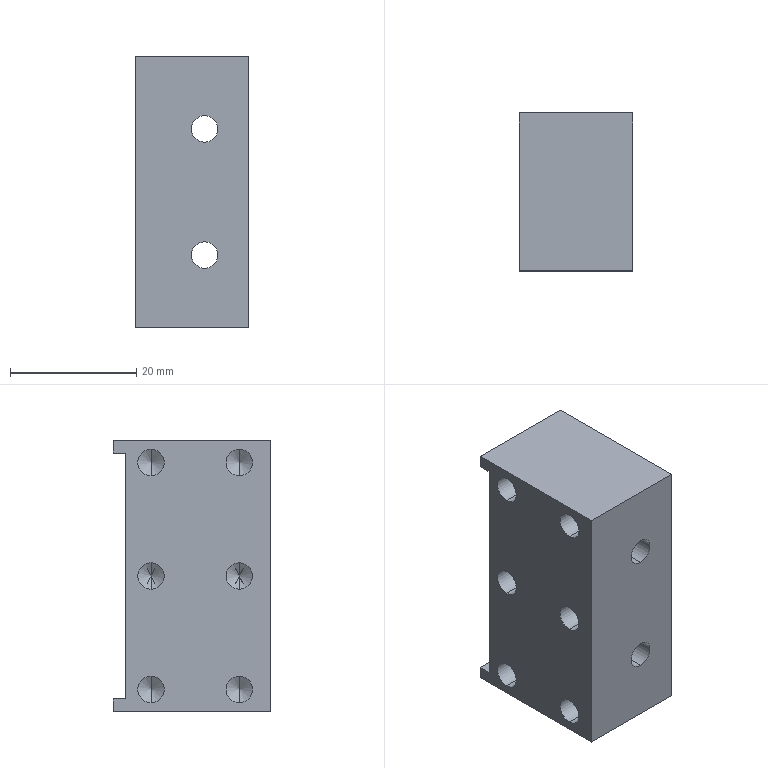Part | NX | features BREP 1 | 1 solid | 38 faces | box 18 x 25 x 43 mm | volume 16077 mm3 | cylinder 16 | cone 12 | plane 10 | commonest cylinder face diameters 4.2 x16
STEP:
#1=CARTESIAN_POINT('',(2.,23.,7.9));
#2=VERTEX_POINT('',#1);
#3=CARTESIAN_POINT('',(2.,0.,7.9));
#4=VERTEX_POINT('',#3);
#5=CARTESIAN_POINT('',(2.,23.,7.9));
#6=DIRECTION('',(0.,1.,0.));
#7=VECTOR('',#6,1000.);
#8=LINE('',#5,#7);
#9=EDGE_CURVE('',#2,#4,#8,.F.);
#10=ORIENTED_EDGE('',*,*,#9,.T.);
#11=CARTESIAN_POINT('',(2.,0.,12.1));
#12=VERTEX_POINT('',#11);
#13=CARTESIAN_POINT('',(2.,0.,10.));
#14=DIRECTION('',(0.,1.,0.));
#15=DIRECTION('',(0.,0.,1.));
#16=AXIS2_PLACEMENT_3D('',#13,#14,#15);
#17=CIRCLE('',#16,2.1);
#18=EDGE_CURVE('',#12,#4,#17,.T.);
#19=ORIENTED_EDGE('',*,*,#18,.F.);
#20=CARTESIAN_POINT('',(2.,23.,12.1));
#21=VERTEX_POINT('',#20);
#22=CARTESIAN_POINT('',(2.,23.,12.1));
#23=DIRECTION('',(0.,1.,0.));
#24=VECTOR('',#23,1000.);
#25=LINE('',#22,#24);
#26=EDGE_CURVE('',#21,#12,#25,.F.);
#27=ORIENTED_EDGE('',*,*,#26,.F.);
#28=CARTESIAN_POINT('',(2.,23.,10.));
#29=DIRECTION('',(0.,1.,0.));
#30=DIRECTION('',(0.,0.,1.));
#31=AXIS2_PLACEMENT_3D('',#28,#29,#30);
#32=CIRCLE('',#31,2.1);
#33=EDGE_CURVE('',#21,#2,#32,.T.);
#34=ORIENTED_EDGE('',*,*,#33,.T.);
#35=EDGE_LOOP('',(#10,#19,#27,#34));
#36=FACE_BOUND('',#35,.T.);
#37=CARTESIAN_POINT('',(2.,23.,10.));
#38=DIRECTION('',(0.,1.,0.));
#39=DIRECTION('',(0.,0.,1.));
#40=AXIS2_PLACEMENT_3D('',#37,#38,#39);
#41=CYLINDRICAL_SURFACE('',#40,2.1);
#42=ADVANCED_FACE('',(#36),#41,.F.);
#43=CARTESIAN_POINT('',(2.,23.,-12.1));
#44=VERTEX_POINT('',#43);
#45=CARTESIAN_POINT('',(2.,0.,-12.1));
#46=VERTEX_POINT('',#45);
#47=CARTESIAN_POINT('',(2.,23.,-12.1));
#48=DIRECTION('',(0.,1.,0.));
#49=VECTOR('',#48,1000.);
#50=LINE('',#47,#49);
#51=EDGE_CURVE('',#44,#46,#50,.F.);
#52=ORIENTED_EDGE('',*,*,#51,.T.);
#53=CARTESIAN_POINT('',(2.,0.,-7.9));
#54=VERTEX_POINT('',#53);
#55=CARTESIAN_POINT('',(2.,0.,-10.));
#56=DIRECTION('',(0.,1.,0.));
#57=DIRECTION('',(0.,0.,1.));
#58=AXIS2_PLACEMENT_3D('',#55,#56,#57);
#59=CIRCLE('',#58,2.1);
#60=EDGE_CURVE('',#54,#46,#59,.T.);
#61=ORIENTED_EDGE('',*,*,#60,.F.);
#62=CARTESIAN_POINT('',(2.,23.,-7.9));
#63=VERTEX_POINT('',#62);
#64=CARTESIAN_POINT('',(2.,23.,-7.9));
#65=DIRECTION('',(0.,1.,0.));
#66=VECTOR('',#65,1000.);
#67=LINE('',#64,#66);
#68=EDGE_CURVE('',#63,#54,#67,.F.);
#69=ORIENTED_EDGE('',*,*,#68,.F.);
#70=CARTESIAN_POINT('',(2.,23.,-10.));
#71=DIRECTION('',(0.,1.,0.));
#72=DIRECTION('',(0.,0.,1.));
#73=AXIS2_PLACEMENT_3D('',#70,#71,#72);
#74=CIRCLE('',#73,2.1);
#75=EDGE_CURVE('',#63,#44,#74,.T.);
#76=ORIENTED_EDGE('',*,*,#75,.T.);
#77=EDGE_LOOP('',(#52,#61,#69,#76));
#78=FACE_BOUND('',#77,.T.);
#79=CARTESIAN_POINT('',(2.,23.,-10.));
#80=DIRECTION('',(0.,1.,0.));
#81=DIRECTION('',(0.,0.,1.));
#82=AXIS2_PLACEMENT_3D('',#79,#80,#81);
#83=CYLINDRICAL_SURFACE('',#82,2.1);
#84=ADVANCED_FACE('',(#78),#83,.F.);
#85=CARTESIAN_POINT('',(-9.,5.,15.9));
#86=VERTEX_POINT('',#85);
#87=CARTESIAN_POINT('',(5.4,5.,15.9));
#88=VERTEX_POINT('',#87);
#89=CARTESIAN_POINT('',(-9.,5.,15.9));
#90=DIRECTION('',(-1.,0.,0.));
#91=VECTOR('',#90,1000.);
#92=LINE('',#89,#91);
#93=EDGE_CURVE('',#86,#88,#92,.F.);
#94=ORIENTED_EDGE('',*,*,#93,.T.);
#95=CARTESIAN_POINT('',(5.4,5.,20.1));
#96=VERTEX_POINT('',#95);
#97=CARTESIAN_POINT('',(5.4,5.,18.));
#98=DIRECTION('',(-1.,0.,0.));
#99=DIRECTION('',(0.,0.,1.));
#100=AXIS2_PLACEMENT_3D('',#97,#98,#99);
#101=CIRCLE('',#100,2.1);
#102=EDGE_CURVE('',#96,#88,#101,.T.);
#103=ORIENTED_EDGE('',*,*,#102,.F.);
#104=CARTESIAN_POINT('',(-9.,5.,20.1));
#105=VERTEX_POINT('',#104);
#106=CARTESIAN_POINT('',(-9.,5.,20.1));
#107=DIRECTION('',(-1.,0.,0.));
#108=VECTOR('',#107,1000.);
#109=LINE('',#106,#108);
#110=EDGE_CURVE('',#105,#96,#109,.F.);
#111=ORIENTED_EDGE('',*,*,#110,.F.);
#112=CARTESIAN_POINT('',(-9.,5.,18.));
#113=DIRECTION('',(-1.,0.,0.));
#114=DIRECTION('',(0.,0.,1.));
#115=AXIS2_PLACEMENT_3D('',#112,#113,#114);
#116=CIRCLE('',#115,2.1);
#117=EDGE_CURVE('',#105,#86,#116,.T.);
#118=ORIENTED_EDGE('',*,*,#117,.T.);
#119=EDGE_LOOP('',(#94,#103,#111,#118));
#120=FACE_BOUND('',#119,.T.);
#121=CARTESIAN_POINT('',(-9.,5.,18.));
#122=DIRECTION('',(-1.,0.,0.));
#123=DIRECTION('',(0.,0.,1.));
#124=AXIS2_PLACEMENT_3D('',#121,#122,#123);
#125=CYLINDRICAL_SURFACE('',#124,2.1);
#126=ADVANCED_FACE('',(#120),#125,.F.);
#127=CARTESIAN_POINT('',(6.662,5.,18.));
#128=VERTEX_POINT('',#127);
#129=CARTESIAN_POINT('',(5.4,5.,15.9));
#130=DIRECTION('',(-0.515,0.,-0.8572));
#131=VECTOR('',#130,1000.);
#132=LINE('',#129,#131);
#133=EDGE_CURVE('',#128,#88,#132,.T.);
#134=ORIENTED_EDGE('',*,*,#133,.F.);
#135=CARTESIAN_POINT('',(5.4,5.,20.1));
#136=DIRECTION('',(-0.515,0.,0.8572));
#137=VECTOR('',#136,1000.);
#138=LINE('',#135,#137);
#139=EDGE_CURVE('',#128,#96,#138,.T.);
#140=ORIENTED_EDGE('',*,*,#139,.T.);
#141=ORIENTED_EDGE('',*,*,#102,.T.);
#142=EDGE_LOOP('',(#134,#140,#141));
#143=FACE_BOUND('',#142,.T.);
#144=CARTESIAN_POINT('',(5.4,5.,18.));
#145=DIRECTION('',(-1.,0.,0.));
#146=DIRECTION('',(0.,0.,1.));
#147=AXIS2_PLACEMENT_3D('',#144,#145,#146);
#148=CONICAL_SURFACE('',#147,2.1,1.03);
#149=ADVANCED_FACE('',(#143),#148,.F.);
#150=CARTESIAN_POINT('',(-9.,5.,-2.1));
#151=VERTEX_POINT('',#150);
#152=CARTESIAN_POINT('',(5.4,5.,-2.1));
#153=VERTEX_POINT('',#152);
#154=CARTESIAN_POINT('',(-9.,5.,-2.1));
#155=DIRECTION('',(-1.,0.,0.));
#156=VECTOR('',#155,1000.);
#157=LINE('',#154,#156);
#158=EDGE_CURVE('',#151,#153,#157,.F.);
#159=ORIENTED_EDGE('',*,*,#158,.T.);
#160=CARTESIAN_POINT('',(5.4,5.,2.1));
#161=VERTEX_POINT('',#160);
#162=CARTESIAN_POINT('',(5.4,5.,0.));
#163=DIRECTION('',(-1.,0.,0.));
#164=DIRECTION('',(0.,0.,1.));
#165=AXIS2_PLACEMENT_3D('',#162,#163,#164);
#166=CIRCLE('',#165,2.1);
#167=EDGE_CURVE('',#161,#153,#166,.T.);
#168=ORIENTED_EDGE('',*,*,#167,.F.);
#169=CARTESIAN_POINT('',(-9.,5.,2.1));
#170=VERTEX_POINT('',#169);
#171=CARTESIAN_POINT('',(-9.,5.,2.1));
#172=DIRECTION('',(-1.,0.,0.));
#173=VECTOR('',#172,1000.);
#174=LINE('',#171,#173);
#175=EDGE_CURVE('',#170,#161,#174,.F.);
#176=ORIENTED_EDGE('',*,*,#175,.F.);
#177=CARTESIAN_POINT('',(-9.,5.,0.));
#178=DIRECTION('',(-1.,0.,0.));
#179=DIRECTION('',(0.,0.,1.));
#180=AXIS2_PLACEMENT_3D('',#177,#178,#179);
#181=CIRCLE('',#180,2.1);
#182=EDGE_CURVE('',#170,#151,#181,.T.);
#183=ORIENTED_EDGE('',*,*,#182,.T.);
#184=EDGE_LOOP('',(#159,#168,#176,#183));
#185=FACE_BOUND('',#184,.T.);
#186=CARTESIAN_POINT('',(-9.,5.,0.));
#187=DIRECTION('',(-1.,0.,0.));
#188=DIRECTION('',(0.,0.,1.));
#189=AXIS2_PLACEMENT_3D('',#186,#187,#188);
#190=CYLINDRICAL_SURFACE('',#189,2.1);
#191=ADVANCED_FACE('',(#185),#190,.F.);
#192=CARTESIAN_POINT('',(6.662,5.,0.));
#193=VERTEX_POINT('',#192);
#194=CARTESIAN_POINT('',(5.4,5.,-2.1));
#195=DIRECTION('',(-0.515,0.,-0.8572));
#196=VECTOR('',#195,1000.);
#197=LINE('',#194,#196);
#198=EDGE_CURVE('',#193,#153,#197,.T.);
#199=ORIENTED_EDGE('',*,*,#198,.F.);
#200=CARTESIAN_POINT('',(5.4,5.,2.1));
#201=DIRECTION('',(-0.515,0.,0.8572));
#202=VECTOR('',#201,1000.);
#203=LINE('',#200,#202);
#204=EDGE_CURVE('',#193,#161,#203,.T.);
#205=ORIENTED_EDGE('',*,*,#204,.T.);
#206=ORIENTED_EDGE('',*,*,#167,.T.);
#207=EDGE_LOOP('',(#199,#205,#206));
#208=FACE_BOUND('',#207,.T.);
#209=CARTESIAN_POINT('',(5.4,5.,0.));
#210=DIRECTION('',(-1.,0.,0.));
#211=DIRECTION('',(0.,0.,1.));
#212=AXIS2_PLACEMENT_3D('',#209,#210,#211);
#213=CONICAL_SURFACE('',#212,2.1,1.03);
#214=ADVANCED_FACE('',(#208),#213,.F.);
#215=CARTESIAN_POINT('',(-9.,5.,-20.1));
#216=VERTEX_POINT('',#215);
#217=CARTESIAN_POINT('',(5.4,5.,-20.1));
#218=VERTEX_POINT('',#217);
#219=CARTESIAN_POINT('',(-9.,5.,-20.1));
#220=DIRECTION('',(-1.,0.,0.));
#221=VECTOR('',#220,1000.);
#222=LINE('',#219,#221);
#223=EDGE_CURVE('',#216,#218,#222,.F.);
#224=ORIENTED_EDGE('',*,*,#223,.T.);
#225=CARTESIAN_POINT('',(5.4,5.,-15.9));
#226=VERTEX_POINT('',#225);
#227=CARTESIAN_POINT('',(5.4,5.,-18.));
#228=DIRECTION('',(-1.,0.,0.));
#229=DIRECTION('',(0.,0.,1.));
#230=AXIS2_PLACEMENT_3D('',#227,#228,#229);
#231=CIRCLE('',#230,2.1);
#232=EDGE_CURVE('',#226,#218,#231,.T.);
#233=ORIENTED_EDGE('',*,*,#232,.F.);
#234=CARTESIAN_POINT('',(-9.,5.,-15.9));
#235=VERTEX_POINT('',#234);
#236=CARTESIAN_POINT('',(-9.,5.,-15.9));
#237=DIRECTION('',(-1.,0.,0.));
#238=VECTOR('',#237,1000.);
#239=LINE('',#236,#238);
#240=EDGE_CURVE('',#235,#226,#239,.F.);
#241=ORIENTED_EDGE('',*,*,#240,.F.);
#242=CARTESIAN_POINT('',(-9.,5.,-18.));
#243=DIRECTION('',(-1.,0.,0.));
#244=DIRECTION('',(0.,0.,1.));
#245=AXIS2_PLACEMENT_3D('',#242,#243,#244);
#246=CIRCLE('',#245,2.1);
#247=EDGE_CURVE('',#235,#216,#246,.T.);
#248=ORIENTED_EDGE('',*,*,#247,.T.);
#249=EDGE_LOOP('',(#224,#233,#241,#248));
#250=FACE_BOUND('',#249,.T.);
#251=CARTESIAN_POINT('',(-9.,5.,-18.));
#252=DIRECTION('',(-1.,0.,0.));
#253=DIRECTION('',(0.,0.,1.));
#254=AXIS2_PLACEMENT_3D('',#251,#252,#253);
#255=CYLINDRICAL_SURFACE('',#254,2.1);
#256=ADVANCED_FACE('',(#250),#255,.F.);
#257=CARTESIAN_POINT('',(6.662,5.,-18.));
#258=VERTEX_POINT('',#257);
#259=CARTESIAN_POINT('',(5.4,5.,-20.1));
#260=DIRECTION('',(-0.515,0.,-0.8572));
#261=VECTOR('',#260,1000.);
#262=LINE('',#259,#261);
#263=EDGE_CURVE('',#258,#218,#262,.T.);
#264=ORIENTED_EDGE('',*,*,#263,.F.);
#265=CARTESIAN_POINT('',(5.4,5.,-15.9));
#266=DIRECTION('',(-0.515,0.,0.8572));
#267=VECTOR('',#266,1000.);
#268=LINE('',#265,#267);
#269=EDGE_CURVE('',#258,#226,#268,.T.);
#270=ORIENTED_EDGE('',*,*,#269,.T.);
#271=ORIENTED_EDGE('',*,*,#232,.T.);
#272=EDGE_LOOP('',(#264,#270,#271));
#273=FACE_BOUND('',#272,.T.);
#274=CARTESIAN_POINT('',(5.4,5.,-18.));
#275=DIRECTION('',(-1.,0.,0.));
#276=DIRECTION('',(0.,0.,1.));
#277=AXIS2_PLACEMENT_3D('',#274,#275,#276);
#278=CONICAL_SURFACE('',#277,2.1,1.03);
#279=ADVANCED_FACE('',(#273),#278,.F.);
#280=CARTESIAN_POINT('',(-9.,19.,15.9));
#281=VERTEX_POINT('',#280);
#282=CARTESIAN_POINT('',(5.4,19.,15.9));
#283=VERTEX_POINT('',#282);
#284=CARTESIAN_POINT('',(-9.,19.,15.9));
#285=DIRECTION('',(-1.,0.,0.));
#286=VECTOR('',#285,1000.);
#287=LINE('',#284,#286);
#288=EDGE_CURVE('',#281,#283,#287,.F.);
#289=ORIENTED_EDGE('',*,*,#288,.T.);
#290=CARTESIAN_POINT('',(5.4,19.,20.1));
#291=VERTEX_POINT('',#290);
#292=CARTESIAN_POINT('',(5.4,19.,18.));
#293=DIRECTION('',(-1.,0.,0.));
#294=DIRECTION('',(0.,0.,1.));
#295=AXIS2_PLACEMENT_3D('',#292,#293,#294);
#296=CIRCLE('',#295,2.1);
#297=EDGE_CURVE('',#291,#283,#296,.T.);
#298=ORIENTED_EDGE('',*,*,#297,.F.);
#299=CARTESIAN_POINT('',(-9.,19.,20.1));
#300=VERTEX_POINT('',#299);
#301=CARTESIAN_POINT('',(-9.,19.,20.1));
#302=DIRECTION('',(-1.,0.,0.));
#303=VECTOR('',#302,1000.);
#304=LINE('',#301,#303);
#305=EDGE_CURVE('',#300,#291,#304,.F.);
#306=ORIENTED_EDGE('',*,*,#305,.F.);
#307=CARTESIAN_POINT('',(-9.,19.,18.));
#308=DIRECTION('',(-1.,0.,0.));
#309=DIRECTION('',(0.,0.,1.));
#310=AXIS2_PLACEMENT_3D('',#307,#308,#309);
#311=CIRCLE('',#310,2.1);
#312=EDGE_CURVE('',#300,#281,#311,.T.);
#313=ORIENTED_EDGE('',*,*,#312,.T.);
#314=EDGE_LOOP('',(#289,#298,#306,#313));
#315=FACE_BOUND('',#314,.T.);
#316=CARTESIAN_POINT('',(-9.,19.,18.));
#317=DIRECTION('',(-1.,0.,0.));
#318=DIRECTION('',(0.,0.,1.));
#319=AXIS2_PLACEMENT_3D('',#316,#317,#318);
#320=CYLINDRICAL_SURFACE('',#319,2.1);
#321=ADVANCED_FACE('',(#315),#320,.F.);
#322=CARTESIAN_POINT('',(6.662,19.,18.));
#323=VERTEX_POINT('',#322);
#324=CARTESIAN_POINT('',(5.4,19.,15.9));
#325=DIRECTION('',(-0.515,0.,-0.8572));
#326=VECTOR('',#325,1000.);
#327=LINE('',#324,#326);
#328=EDGE_CURVE('',#323,#283,#327,.T.);
#329=ORIENTED_EDGE('',*,*,#328,.F.);
#330=CARTESIAN_POINT('',(5.4,19.,20.1));
#331=DIRECTION('',(-0.515,0.,0.8572));
#332=VECTOR('',#331,1000.);
#333=LINE('',#330,#332);
#334=EDGE_CURVE('',#323,#291,#333,.T.);
#335=ORIENTED_EDGE('',*,*,#334,.T.);
#336=ORIENTED_EDGE('',*,*,#297,.T.);
#337=EDGE_LOOP('',(#329,#335,#336));
#338=FACE_BOUND('',#337,.T.);
#339=CARTESIAN_POINT('',(5.4,19.,18.));
#340=DIRECTION('',(-1.,0.,0.));
#341=DIRECTION('',(0.,0.,1.));
#342=AXIS2_PLACEMENT_3D('',#339,#340,#341);
#343=CONICAL_SURFACE('',#342,2.1,1.03);
#344=ADVANCED_FACE('',(#338),#343,.F.);
#345=CARTESIAN_POINT('',(-9.,19.,-2.1));
#346=VERTEX_POINT('',#345);
#347=CARTESIAN_POINT('',(5.4,19.,-2.1));
#348=VERTEX_POINT('',#347);
#349=CARTESIAN_POINT('',(-9.,19.,-2.1));
#350=DIRECTION('',(-1.,0.,0.));
#351=VECTOR('',#350,1000.);
#352=LINE('',#349,#351);
#353=EDGE_CURVE('',#346,#348,#352,.F.);
#354=ORIENTED_EDGE('',*,*,#353,.T.);
#355=CARTESIAN_POINT('',(5.4,19.,2.1));
#356=VERTEX_POINT('',#355);
#357=CARTESIAN_POINT('',(5.4,19.,0.));
#358=DIRECTION('',(-1.,0.,0.));
#359=DIRECTION('',(0.,0.,1.));
#360=AXIS2_PLACEMENT_3D('',#357,#358,#359);
#361=CIRCLE('',#360,2.1);
#362=EDGE_CURVE('',#356,#348,#361,.T.);
#363=ORIENTED_EDGE('',*,*,#362,.F.);
#364=CARTESIAN_POINT('',(-9.,19.,2.1));
#365=VERTEX_POINT('',#364);
#366=CARTESIAN_POINT('',(-9.,19.,2.1));
#367=DIRECTION('',(-1.,0.,0.));
#368=VECTOR('',#367,1000.);
#369=LINE('',#366,#368);
#370=EDGE_CURVE('',#365,#356,#369,.F.);
#371=ORIENTED_EDGE('',*,*,#370,.F.);
#372=CARTESIAN_POINT('',(-9.,19.,0.));
#373=DIRECTION('',(-1.,0.,0.));
#374=DIRECTION('',(0.,0.,1.));
#375=AXIS2_PLACEMENT_3D('',#372,#373,#374);
#376=CIRCLE('',#375,2.1);
#377=EDGE_CURVE('',#365,#346,#376,.T.);
#378=ORIENTED_EDGE('',*,*,#377,.T.);
#379=EDGE_LOOP('',(#354,#363,#371,#378));
#380=FACE_BOUND('',#379,.T.);
#381=CARTESIAN_POINT('',(-9.,19.,0.));
#382=DIRECTION('',(-1.,0.,0.));
#383=DIRECTION('',(0.,0.,1.));
#384=AXIS2_PLACEMENT_3D('',#381,#382,#383);
#385=CYLINDRICAL_SURFACE('',#384,2.1);
#386=ADVANCED_FACE('',(#380),#385,.F.);
#387=CARTESIAN_POINT('',(6.662,19.,0.));
#388=VERTEX_POINT('',#387);
#389=CARTESIAN_POINT('',(5.4,19.,-2.1));
#390=DIRECTION('',(-0.515,0.,-0.8572));
#391=VECTOR('',#390,1000.);
#392=LINE('',#389,#391);
#393=EDGE_CURVE('',#388,#348,#392,.T.);
#394=ORIENTED_EDGE('',*,*,#393,.F.);
#395=CARTESIAN_POINT('',(5.4,19.,2.1));
#396=DIRECTION('',(-0.515,0.,0.8572));
#397=VECTOR('',#396,1000.);
#398=LINE('',#395,#397);
#399=EDGE_CURVE('',#388,#356,#398,.T.);
#400=ORIENTED_EDGE('',*,*,#399,.T.);
#401=ORIENTED_EDGE('',*,*,#362,.T.);
#402=EDGE_LOOP('',(#394,#400,#401));
#403=FACE_BOUND('',#402,.T.);
#404=CARTESIAN_POINT('',(5.4,19.,0.));
#405=DIRECTION('',(-1.,0.,0.));
#406=DIRECTION('',(0.,0.,1.));
#407=AXIS2_PLACEMENT_3D('',#404,#405,#406);
#408=CONICAL_SURFACE('',#407,2.1,1.03);
#409=ADVANCED_FACE('',(#403),#408,.F.);
#410=CARTESIAN_POINT('',(-9.,19.,-20.1));
#411=VERTEX_POINT('',#410);
#412=CARTESIAN_POINT('',(5.4,19.,-20.1));
#413=VERTEX_POINT('',#412);
#414=CARTESIAN_POINT('',(-9.,19.,-20.1));
#415=DIRECTION('',(-1.,0.,0.));
#416=VECTOR('',#415,1000.);
#417=LINE('',#414,#416);
#418=EDGE_CURVE('',#411,#413,#417,.F.);
#419=ORIENTED_EDGE('',*,*,#418,.T.);
#420=CARTESIAN_POINT('',(5.4,19.,-15.9));
#421=VERTEX_POINT('',#420);
#422=CARTESIAN_POINT('',(5.4,19.,-18.));
#423=DIRECTION('',(-1.,0.,0.));
#424=DIRECTION('',(0.,0.,1.));
#425=AXIS2_PLACEMENT_3D('',#422,#423,#424);
#426=CIRCLE('',#425,2.1);
#427=EDGE_CURVE('',#421,#413,#426,.T.);
#428=ORIENTED_EDGE('',*,*,#427,.F.);
#429=CARTESIAN_POINT('',(-9.,19.,-15.9));
#430=VERTEX_POINT('',#429);
#431=CARTESIAN_POINT('',(-9.,19.,-15.9));
#432=DIRECTION('',(-1.,0.,0.));
#433=VECTOR('',#432,1000.);
#434=LINE('',#431,#433);
#435=EDGE_CURVE('',#430,#421,#434,.F.);
#436=ORIENTED_EDGE('',*,*,#435,.F.);
#437=CARTESIAN_POINT('',(-9.,19.,-18.));
#438=DIRECTION('',(-1.,0.,0.));
#439=DIRECTION('',(0.,0.,1.));
#440=AXIS2_PLACEMENT_3D('',#437,#438,#439);
#441=CIRCLE('',#440,2.1);
#442=EDGE_CURVE('',#430,#411,#441,.T.);
#443=ORIENTED_EDGE('',*,*,#442,.T.);
#444=EDGE_LOOP('',(#419,#428,#436,#443));
#445=FACE_BOUND('',#444,.T.);
#446=CARTESIAN_POINT('',(-9.,19.,-18.));
#447=DIRECTION('',(-1.,0.,0.));
#448=DIRECTION('',(0.,0.,1.));
#449=AXIS2_PLACEMENT_3D('',#446,#447,#448);
#450=CYLINDRICAL_SURFACE('',#449,2.1);
#451=ADVANCED_FACE('',(#445),#450,.F.);
#452=CARTESIAN_POINT('',(6.662,19.,-18.));
#453=VERTEX_POINT('',#452);
#454=CARTESIAN_POINT('',(5.4,19.,-20.1));
#455=DIRECTION('',(-0.515,0.,-0.8572));
#456=VECTOR('',#455,1000.);
#457=LINE('',#454,#456);
#458=EDGE_CURVE('',#453,#413,#457,.T.);
#459=ORIENTED_EDGE('',*,*,#458,.F.);
#460=CARTESIAN_POINT('',(5.4,19.,-15.9));
#461=DIRECTION('',(-0.515,0.,0.8572));
#462=VECTOR('',#461,1000.);
#463=LINE('',#460,#462);
#464=EDGE_CURVE('',#453,#421,#463,.T.);
#465=ORIENTED_EDGE('',*,*,#464,.T.);
#466=ORIENTED_EDGE('',*,*,#427,.T.);
#467=EDGE_LOOP('',(#459,#465,#466));
#468=FACE_BOUND('',#467,.T.);
#469=CARTESIAN_POINT('',(5.4,19.,-18.));
#470=DIRECTION('',(-1.,0.,0.));
#471=DIRECTION('',(0.,0.,1.));
#472=AXIS2_PLACEMENT_3D('',#469,#470,#471);
#473=CONICAL_SURFACE('',#472,2.1,1.03);
#474=ADVANCED_FACE('',(#468),#473,.F.);
#475=CARTESIAN_POINT('',(-9.,23.,-19.5));
#476=VERTEX_POINT('',#475);
#477=CARTESIAN_POINT('',(-9.,23.,19.5));
#478=VERTEX_POINT('',#477);
#479=CARTESIAN_POINT('',(-9.,23.,19.5));
#480=DIRECTION('',(0.,0.,1.));
#481=VECTOR('',#480,1000.);
#482=LINE('',#479,#481);
#483=EDGE_CURVE('',#476,#478,#482,.T.);
#484=ORIENTED_EDGE('',*,*,#483,.T.);
#485=CARTESIAN_POINT('',(9.,23.,19.5));
#486=VERTEX_POINT('',#485);
#487=CARTESIAN_POINT('',(9.,23.,19.5));
#488=DIRECTION('',(1.,0.,0.));
#489=VECTOR('',#488,1000.);
#490=LINE('',#487,#489);
#491=EDGE_CURVE('',#478,#486,#490,.T.);
#492=ORIENTED_EDGE('',*,*,#491,.T.);
#493=CARTESIAN_POINT('',(9.,23.,-19.5));
#494=VERTEX_POINT('',#493);
#495=CARTESIAN_POINT('',(9.,23.,19.5));
#496=DIRECTION('',(0.,0.,-1.));
#497=VECTOR('',#496,1000.);
#498=LINE('',#495,#497);
#499=EDGE_CURVE('',#486,#494,#498,.T.);
#500=ORIENTED_EDGE('',*,*,#499,.T.);
#501=CARTESIAN_POINT('',(9.,23.,-19.5));
#502=DIRECTION('',(-1.,0.,0.));
#503=VECTOR('',#502,1000.);
#504=LINE('',#501,#503);
#505=EDGE_CURVE('',#494,#476,#504,.T.);
#506=ORIENTED_EDGE('',*,*,#505,.T.);
#507=EDGE_LOOP('',(#484,#492,#500,#506));
#508=FACE_BOUND('',#507,.T.);
#509=ORIENTED_EDGE('',*,*,#75,.F.);
#510=CARTESIAN_POINT('',(2.,23.,-10.));
#511=DIRECTION('',(0.,1.,0.));
#512=DIRECTION('',(0.,0.,1.));
#513=AXIS2_PLACEMENT_3D('',#510,#511,#512);
#514=CIRCLE('',#513,2.1);
#515=EDGE_CURVE('',#44,#63,#514,.T.);
#516=ORIENTED_EDGE('',*,*,#515,.F.);
#517=EDGE_LOOP('',(#509,#516));
#518=FACE_BOUND('',#517,.T.);
#519=ORIENTED_EDGE('',*,*,#33,.F.);
#520=CARTESIAN_POINT('',(2.,23.,10.));
#521=DIRECTION('',(0.,1.,0.));
#522=DIRECTION('',(0.,0.,1.));
#523=AXIS2_PLACEMENT_3D('',#520,#521,#522);
#524=CIRCLE('',#523,2.1);
#525=EDGE_CURVE('',#2,#21,#524,.T.);
#526=ORIENTED_EDGE('',*,*,#525,.F.);
#527=EDGE_LOOP('',(#519,#526));
#528=FACE_BOUND('',#527,.T.);
#529=CARTESIAN_POINT('',(0.,23.,0.));
#530=DIRECTION('',(0.,1.,0.));
#531=DIRECTION('',(0.,0.,1.));
#532=AXIS2_PLACEMENT_3D('',#529,#530,#531);
#533=PLANE('',#532);
#534=ADVANCED_FACE('',(#508,#518,#528),#533,.T.);
#535=CARTESIAN_POINT('',(-9.,25.,19.5));
#536=VERTEX_POINT('',#535);
#537=CARTESIAN_POINT('',(9.,25.,19.5));
#538=VERTEX_POINT('',#537);
#539=CARTESIAN_POINT('',(9.,25.,19.5));
#540=DIRECTION('',(1.,0.,0.));
#541=VECTOR('',#540,1000.);
#542=LINE('',#539,#541);
#543=EDGE_CURVE('',#536,#538,#542,.T.);
#544=ORIENTED_EDGE('',*,*,#543,.T.);
#545=CARTESIAN_POINT('',(9.,23.,19.5));
#546=DIRECTION('',(0.,1.,0.));
#547=VECTOR('',#546,1000.);
#548=LINE('',#545,#547);
#549=EDGE_CURVE('',#486,#538,#548,.T.);
#550=ORIENTED_EDGE('',*,*,#549,.F.);
#551=ORIENTED_EDGE('',*,*,#491,.F.);
#552=CARTESIAN_POINT('',(-9.,23.,19.5));
#553=DIRECTION('',(0.,1.,0.));
#554=VECTOR('',#553,1000.);
#555=LINE('',#552,#554);
#556=EDGE_CURVE('',#478,#536,#555,.T.);
#557=ORIENTED_EDGE('',*,*,#556,.T.);
#558=EDGE_LOOP('',(#544,#550,#551,#557));
#559=FACE_BOUND('',#558,.T.);
#560=CARTESIAN_POINT('',(9.,23.,19.5));
#561=DIRECTION('',(0.,0.,1.));
#562=DIRECTION('',(1.,0.,0.));
#563=AXIS2_PLACEMENT_3D('',#560,#561,#562);
#564=PLANE('',#563);
#565=ADVANCED_FACE('',(#559),#564,.F.);
#566=CARTESIAN_POINT('',(9.,25.,-19.5));
#567=VERTEX_POINT('',#566);
#568=CARTESIAN_POINT('',(-9.,25.,-19.5));
#569=VERTEX_POINT('',#568);
#570=CARTESIAN_POINT('',(9.,25.,-19.5));
#571=DIRECTION('',(-1.,0.,0.));
#572=VECTOR('',#571,1000.);
#573=LINE('',#570,#572);
#574=EDGE_CURVE('',#567,#569,#573,.T.);
#575=ORIENTED_EDGE('',*,*,#574,.T.);
#576=CARTESIAN_POINT('',(-9.,23.,-19.5));
#577=DIRECTION('',(0.,1.,0.));
#578=VECTOR('',#577,1000.);
#579=LINE('',#576,#578);
#580=EDGE_CURVE('',#476,#569,#579,.T.);
#581=ORIENTED_EDGE('',*,*,#580,.F.);
#582=ORIENTED_EDGE('',*,*,#505,.F.);
#583=CARTESIAN_POINT('',(9.,23.,-19.5));
#584=DIRECTION('',(0.,1.,0.));
#585=VECTOR('',#584,1000.);
#586=LINE('',#583,#585);
#587=EDGE_CURVE('',#494,#567,#586,.T.);
#588=ORIENTED_EDGE('',*,*,#587,.T.);
#589=EDGE_LOOP('',(#575,#581,#582,#588));
#590=FACE_BOUND('',#589,.T.);
#591=CARTESIAN_POINT('',(9.,23.,-19.5));
#592=DIRECTION('',(0.,0.,-1.));
#593=DIRECTION('',(-1.,0.,0.));
#594=AXIS2_PLACEMENT_3D('',#591,#592,#593);
#595=PLANE('',#594);
#596=ADVANCED_FACE('',(#590),#595,.F.);
#597=CARTESIAN_POINT('',(9.,0.,21.5));
#598=VERTEX_POINT('',#597);
#599=CARTESIAN_POINT('',(9.,0.,-21.5));
#600=VERTEX_POINT('',#599);
#601=CARTESIAN_POINT('',(9.,0.,21.5));
#602=DIRECTION('',(0.,0.,-1.));
#603=VECTOR('',#602,1000.);
#604=LINE('',#601,#603);
#605=EDGE_CURVE('',#598,#600,#604,.T.);
#606=ORIENTED_EDGE('',*,*,#605,.F.);
#607=CARTESIAN_POINT('',(-9.,0.,21.5));
#608=VERTEX_POINT('',#607);
#609=CARTESIAN_POINT('',(-9.,0.,21.5));
#610=DIRECTION('',(1.,0.,0.));
#611=VECTOR('',#610,1000.);
#612=LINE('',#609,#611);
#613=EDGE_CURVE('',#608,#598,#612,.T.);
#614=ORIENTED_EDGE('',*,*,#613,.F.);
#615=CARTESIAN_POINT('',(-9.,0.,-21.5));
#616=VERTEX_POINT('',#615);
#617=CARTESIAN_POINT('',(-9.,0.,21.5));
#618=DIRECTION('',(0.,0.,1.));
#619=VECTOR('',#618,1000.);
#620=LINE('',#617,#619);
#621=EDGE_CURVE('',#616,#608,#620,.T.);
#622=ORIENTED_EDGE('',*,*,#621,.F.);
#623=CARTESIAN_POINT('',(-9.,0.,-21.5));
#624=DIRECTION('',(-1.,0.,0.));
#625=VECTOR('',#624,1000.);
#626=LINE('',#623,#625);
#627=EDGE_CURVE('',#600,#616,#626,.T.);
#628=ORIENTED_EDGE('',*,*,#627,.F.);
#629=EDGE_LOOP('',(#606,#614,#622,#628));
#630=FACE_BOUND('',#629,.T.);
#631=ORIENTED_EDGE('',*,*,#60,.T.);
#632=CARTESIAN_POINT('',(2.,0.,-10.));
#633=DIRECTION('',(0.,1.,0.));
#634=DIRECTION('',(0.,0.,1.));
#635=AXIS2_PLACEMENT_3D('',#632,#633,#634);
#636=CIRCLE('',#635,2.1);
#637=EDGE_CURVE('',#46,#54,#636,.T.);
#638=ORIENTED_EDGE('',*,*,#637,.T.);
#639=EDGE_LOOP('',(#631,#638));
#640=FACE_BOUND('',#639,.T.);
#641=ORIENTED_EDGE('',*,*,#18,.T.);
#642=CARTESIAN_POINT('',(2.,0.,10.));
#643=DIRECTION('',(0.,1.,0.));
#644=DIRECTION('',(0.,0.,1.));
#645=AXIS2_PLACEMENT_3D('',#642,#643,#644);
#646=CIRCLE('',#645,2.1);
#647=EDGE_CURVE('',#4,#12,#646,.T.);
#648=ORIENTED_EDGE('',*,*,#647,.T.);
#649=EDGE_LOOP('',(#641,#648));
#650=FACE_BOUND('',#649,.T.);
#651=CARTESIAN_POINT('',(0.,0.,0.));
#652=DIRECTION('',(0.,-1.,0.));
#653=DIRECTION('',(0.,0.,-1.));
#654=AXIS2_PLACEMENT_3D('',#651,#652,#653);
#655=PLANE('',#654);
#656=ADVANCED_FACE('',(#630,#640,#650),#655,.T.);
#657=CARTESIAN_POINT('',(9.,25.,21.5));
#658=VERTEX_POINT('',#657);
#659=CARTESIAN_POINT('',(9.,25.,21.5));
#660=DIRECTION('',(0.,0.,-1.));
#661=VECTOR('',#660,1000.);
#662=LINE('',#659,#661);
#663=EDGE_CURVE('',#658,#538,#662,.T.);
#664=ORIENTED_EDGE('',*,*,#663,.T.);
#665=ORIENTED_EDGE('',*,*,#543,.F.);
#666=CARTESIAN_POINT('',(-9.,25.,21.5));
#667=VERTEX_POINT('',#666);
#668=CARTESIAN_POINT('',(-9.,25.,21.5));
#669=DIRECTION('',(0.,0.,1.));
#670=VECTOR('',#669,1000.);
#671=LINE('',#668,#670);
#672=EDGE_CURVE('',#536,#667,#671,.T.);
#673=ORIENTED_EDGE('',*,*,#672,.T.);
#674=CARTESIAN_POINT('',(-9.,25.,21.5));
#675=DIRECTION('',(1.,0.,0.));
#676=VECTOR('',#675,1000.);
#677=LINE('',#674,#676);
#678=EDGE_CURVE('',#667,#658,#677,.T.);
#679=ORIENTED_EDGE('',*,*,#678,.T.);
#680=EDGE_LOOP('',(#664,#665,#673,#679));
#681=FACE_BOUND('',#680,.T.);
#682=CARTESIAN_POINT('',(0.,25.,0.));
#683=DIRECTION('',(0.,-1.,0.));
#684=DIRECTION('',(0.,0.,-1.));
#685=AXIS2_PLACEMENT_3D('',#682,#683,#684);
#686=PLANE('',#685);
#687=ADVANCED_FACE('',(#681),#686,.F.);
#688=ORIENTED_EDGE('',*,*,#613,.T.);
#689=CARTESIAN_POINT('',(9.,25.,21.5));
#690=DIRECTION('',(0.,-1.,0.));
#691=VECTOR('',#690,1000.);
#692=LINE('',#689,#691);
#693=EDGE_CURVE('',#658,#598,#692,.T.);
#694=ORIENTED_EDGE('',*,*,#693,.F.);
#695=ORIENTED_EDGE('',*,*,#678,.F.);
#696=CARTESIAN_POINT('',(-9.,25.,21.5));
#697=DIRECTION('',(0.,-1.,0.));
#698=VECTOR('',#697,1000.);
#699=LINE('',#696,#698);
#700=EDGE_CURVE('',#667,#608,#699,.T.);
#701=ORIENTED_EDGE('',*,*,#700,.T.);
#702=EDGE_LOOP('',(#688,#694,#695,#701));
#703=FACE_BOUND('',#702,.T.);
#704=CARTESIAN_POINT('',(-9.,25.,21.5));
#705=DIRECTION('',(0.,0.,-1.));
#706=DIRECTION('',(-1.,0.,0.));
#707=AXIS2_PLACEMENT_3D('',#704,#705,#706);
#708=PLANE('',#707);
#709=ADVANCED_FACE('',(#703),#708,.F.);
#710=ORIENTED_EDGE('',*,*,#483,.F.);
#711=ORIENTED_EDGE('',*,*,#580,.T.);
#712=CARTESIAN_POINT('',(-9.,25.,-21.5));
#713=VERTEX_POINT('',#712);
#714=CARTESIAN_POINT('',(-9.,25.,21.5));
#715=DIRECTION('',(0.,0.,1.));
#716=VECTOR('',#715,1000.);
#717=LINE('',#714,#716);
#718=EDGE_CURVE('',#713,#569,#717,.T.);
#719=ORIENTED_EDGE('',*,*,#718,.F.);
#720=CARTESIAN_POINT('',(-9.,25.,-21.5));
#721=DIRECTION('',(0.,-1.,0.));
#722=VECTOR('',#721,1000.);
#723=LINE('',#720,#722);
#724=EDGE_CURVE('',#713,#616,#723,.T.);
#725=ORIENTED_EDGE('',*,*,#724,.T.);
#726=ORIENTED_EDGE('',*,*,#621,.T.);
#727=ORIENTED_EDGE('',*,*,#700,.F.);
#728=ORIENTED_EDGE('',*,*,#672,.F.);
#729=ORIENTED_EDGE('',*,*,#556,.F.);
#730=EDGE_LOOP('',(#710,#711,#719,#725,#726,#727,#728,#729));
#731=FACE_BOUND('',#730,.T.);
#732=ORIENTED_EDGE('',*,*,#442,.F.);
#733=CARTESIAN_POINT('',(-9.,19.,-18.));
#734=DIRECTION('',(-1.,0.,0.));
#735=DIRECTION('',(0.,0.,1.));
#736=AXIS2_PLACEMENT_3D('',#733,#734,#735);
#737=CIRCLE('',#736,2.1);
#738=EDGE_CURVE('',#411,#430,#737,.T.);
#739=ORIENTED_EDGE('',*,*,#738,.F.);
#740=EDGE_LOOP('',(#732,#739));
#741=FACE_BOUND('',#740,.T.);
#742=ORIENTED_EDGE('',*,*,#377,.F.);
#743=CARTESIAN_POINT('',(-9.,19.,0.));
#744=DIRECTION('',(-1.,0.,0.));
#745=DIRECTION('',(0.,0.,1.));
#746=AXIS2_PLACEMENT_3D('',#743,#744,#745);
#747=CIRCLE('',#746,2.1);
#748=EDGE_CURVE('',#346,#365,#747,.T.);
#749=ORIENTED_EDGE('',*,*,#748,.F.);
#750=EDGE_LOOP('',(#742,#749));
#751=FACE_BOUND('',#750,.T.);
#752=ORIENTED_EDGE('',*,*,#312,.F.);
#753=CARTESIAN_POINT('',(-9.,19.,18.));
#754=DIRECTION('',(-1.,0.,0.));
#755=DIRECTION('',(0.,0.,1.));
#756=AXIS2_PLACEMENT_3D('',#753,#754,#755);
#757=CIRCLE('',#756,2.1);
#758=EDGE_CURVE('',#281,#300,#757,.T.);
#759=ORIENTED_EDGE('',*,*,#758,.F.);
#760=EDGE_LOOP('',(#752,#759));
#761=FACE_BOUND('',#760,.T.);
#762=ORIENTED_EDGE('',*,*,#247,.F.);
#763=CARTESIAN_POINT('',(-9.,5.,-18.));
#764=DIRECTION('',(-1.,0.,0.));
#765=DIRECTION('',(0.,0.,1.));
#766=AXIS2_PLACEMENT_3D('',#763,#764,#765);
#767=CIRCLE('',#766,2.1);
#768=EDGE_CURVE('',#216,#235,#767,.T.);
#769=ORIENTED_EDGE('',*,*,#768,.F.);
#770=EDGE_LOOP('',(#762,#769));
#771=FACE_BOUND('',#770,.T.);
#772=ORIENTED_EDGE('',*,*,#182,.F.);
#773=CARTESIAN_POINT('',(-9.,5.,0.));
#774=DIRECTION('',(-1.,0.,0.));
#775=DIRECTION('',(0.,0.,1.));
#776=AXIS2_PLACEMENT_3D('',#773,#774,#775);
#777=CIRCLE('',#776,2.1);
#778=EDGE_CURVE('',#151,#170,#777,.T.);
#779=ORIENTED_EDGE('',*,*,#778,.F.);
#780=EDGE_LOOP('',(#772,#779));
#781=FACE_BOUND('',#780,.T.);
#782=ORIENTED_EDGE('',*,*,#117,.F.);
#783=CARTESIAN_POINT('',(-9.,5.,18.));
#784=DIRECTION('',(-1.,0.,0.));
#785=DIRECTION('',(0.,0.,1.));
#786=AXIS2_PLACEMENT_3D('',#783,#784,#785);
#787=CIRCLE('',#786,2.1);
#788=EDGE_CURVE('',#86,#105,#787,.T.);
#789=ORIENTED_EDGE('',*,*,#788,.F.);
#790=EDGE_LOOP('',(#782,#789));
#791=FACE_BOUND('',#790,.T.);
#792=CARTESIAN_POINT('',(-9.,25.,21.5));
#793=DIRECTION('',(1.,0.,0.));
#794=DIRECTION('',(0.,0.,-1.));
#795=AXIS2_PLACEMENT_3D('',#792,#793,#794);
#796=PLANE('',#795);
#797=ADVANCED_FACE('',(#731,#741,#751,#761,#771,#781,#791),#796,.F.);
#798=ORIENTED_EDGE('',*,*,#627,.T.);
#799=ORIENTED_EDGE('',*,*,#724,.F.);
#800=CARTESIAN_POINT('',(9.,25.,-21.5));
#801=VERTEX_POINT('',#800);
#802=CARTESIAN_POINT('',(-9.,25.,-21.5));
#803=DIRECTION('',(-1.,0.,0.));
#804=VECTOR('',#803,1000.);
#805=LINE('',#802,#804);
#806=EDGE_CURVE('',#801,#713,#805,.T.);
#807=ORIENTED_EDGE('',*,*,#806,.F.);
#808=CARTESIAN_POINT('',(9.,25.,-21.5));
#809=DIRECTION('',(0.,-1.,0.));
#810=VECTOR('',#809,1000.);
#811=LINE('',#808,#810);
#812=EDGE_CURVE('',#801,#600,#811,.T.);
#813=ORIENTED_EDGE('',*,*,#812,.T.);
#814=EDGE_LOOP('',(#798,#799,#807,#813));
#815=FACE_BOUND('',#814,.T.);
#816=CARTESIAN_POINT('',(-9.,25.,-21.5));
#817=DIRECTION('',(0.,0.,1.));
#818=DIRECTION('',(1.,0.,0.));
#819=AXIS2_PLACEMENT_3D('',#816,#817,#818);
#820=PLANE('',#819);
#821=ADVANCED_FACE('',(#815),#820,.F.);
#822=CARTESIAN_POINT('',(9.,25.,21.5));
#823=DIRECTION('',(0.,0.,-1.));
#824=VECTOR('',#823,1000.);
#825=LINE('',#822,#824);
#826=EDGE_CURVE('',#567,#801,#825,.T.);
#827=ORIENTED_EDGE('',*,*,#826,.F.);
#828=ORIENTED_EDGE('',*,*,#587,.F.);
#829=ORIENTED_EDGE('',*,*,#499,.F.);
#830=ORIENTED_EDGE('',*,*,#549,.T.);
#831=ORIENTED_EDGE('',*,*,#663,.F.);
#832=ORIENTED_EDGE('',*,*,#693,.T.);
#833=ORIENTED_EDGE('',*,*,#605,.T.);
#834=ORIENTED_EDGE('',*,*,#812,.F.);
#835=EDGE_LOOP('',(#827,#828,#829,#830,#831,#832,#833,#834));
#836=FACE_BOUND('',#835,.T.);
#837=CARTESIAN_POINT('',(9.,25.,21.5));
#838=DIRECTION('',(-1.,0.,0.));
#839=DIRECTION('',(0.,0.,1.));
#840=AXIS2_PLACEMENT_3D('',#837,#838,#839);
#841=PLANE('',#840);
#842=ADVANCED_FACE('',(#836),#841,.F.);
#843=ORIENTED_EDGE('',*,*,#718,.T.);
#844=ORIENTED_EDGE('',*,*,#574,.F.);
#845=ORIENTED_EDGE('',*,*,#826,.T.);
#846=ORIENTED_EDGE('',*,*,#806,.T.);
#847=EDGE_LOOP('',(#843,#844,#845,#846));
#848=FACE_BOUND('',#847,.T.);
#849=CARTESIAN_POINT('',(0.,25.,0.));
#850=DIRECTION('',(0.,-1.,0.));
#851=DIRECTION('',(0.,0.,-1.));
#852=AXIS2_PLACEMENT_3D('',#849,#850,#851);
#853=PLANE('',#852);
#854=ADVANCED_FACE('',(#848),#853,.F.);
#855=ORIENTED_EDGE('',*,*,#464,.F.);
#856=ORIENTED_EDGE('',*,*,#458,.T.);
#857=CARTESIAN_POINT('',(5.4,19.,-18.));
#858=DIRECTION('',(-1.,0.,0.));
#859=DIRECTION('',(0.,0.,1.));
#860=AXIS2_PLACEMENT_3D('',#857,#858,#859);
#861=CIRCLE('',#860,2.1);
#862=EDGE_CURVE('',#413,#421,#861,.T.);
#863=ORIENTED_EDGE('',*,*,#862,.T.);
#864=EDGE_LOOP('',(#855,#856,#863));
#865=FACE_BOUND('',#864,.T.);
#866=CARTESIAN_POINT('',(5.4,19.,-18.));
#867=DIRECTION('',(-1.,0.,0.));
#868=DIRECTION('',(0.,0.,1.));
#869=AXIS2_PLACEMENT_3D('',#866,#867,#868);
#870=CONICAL_SURFACE('',#869,2.1,1.03);
#871=ADVANCED_FACE('',(#865),#870,.F.);
#872=ORIENTED_EDGE('',*,*,#862,.F.);
#873=ORIENTED_EDGE('',*,*,#418,.F.);
#874=ORIENTED_EDGE('',*,*,#738,.T.);
#875=ORIENTED_EDGE('',*,*,#435,.T.);
#876=EDGE_LOOP('',(#872,#873,#874,#875));
#877=FACE_BOUND('',#876,.T.);
#878=CARTESIAN_POINT('',(-9.,19.,-18.));
#879=DIRECTION('',(-1.,0.,0.));
#880=DIRECTION('',(0.,0.,1.));
#881=AXIS2_PLACEMENT_3D('',#878,#879,#880);
#882=CYLINDRICAL_SURFACE('',#881,2.1);
#883=ADVANCED_FACE('',(#877),#882,.F.);
#884=ORIENTED_EDGE('',*,*,#399,.F.);
#885=ORIENTED_EDGE('',*,*,#393,.T.);
#886=CARTESIAN_POINT('',(5.4,19.,0.));
#887=DIRECTION('',(-1.,0.,0.));
#888=DIRECTION('',(0.,0.,1.));
#889=AXIS2_PLACEMENT_3D('',#886,#887,#888);
#890=CIRCLE('',#889,2.1);
#891=EDGE_CURVE('',#348,#356,#890,.T.);
#892=ORIENTED_EDGE('',*,*,#891,.T.);
#893=EDGE_LOOP('',(#884,#885,#892));
#894=FACE_BOUND('',#893,.T.);
#895=CARTESIAN_POINT('',(5.4,19.,0.));
#896=DIRECTION('',(-1.,0.,0.));
#897=DIRECTION('',(0.,0.,1.));
#898=AXIS2_PLACEMENT_3D('',#895,#896,#897);
#899=CONICAL_SURFACE('',#898,2.1,1.03);
#900=ADVANCED_FACE('',(#894),#899,.F.);
#901=ORIENTED_EDGE('',*,*,#891,.F.);
#902=ORIENTED_EDGE('',*,*,#353,.F.);
#903=ORIENTED_EDGE('',*,*,#748,.T.);
#904=ORIENTED_EDGE('',*,*,#370,.T.);
#905=EDGE_LOOP('',(#901,#902,#903,#904));
#906=FACE_BOUND('',#905,.T.);
#907=CARTESIAN_POINT('',(-9.,19.,0.));
#908=DIRECTION('',(-1.,0.,0.));
#909=DIRECTION('',(0.,0.,1.));
#910=AXIS2_PLACEMENT_3D('',#907,#908,#909);
#911=CYLINDRICAL_SURFACE('',#910,2.1);
#912=ADVANCED_FACE('',(#906),#911,.F.);
#913=ORIENTED_EDGE('',*,*,#334,.F.);
#914=ORIENTED_EDGE('',*,*,#328,.T.);
#915=CARTESIAN_POINT('',(5.4,19.,18.));
#916=DIRECTION('',(-1.,0.,0.));
#917=DIRECTION('',(0.,0.,1.));
#918=AXIS2_PLACEMENT_3D('',#915,#916,#917);
#919=CIRCLE('',#918,2.1);
#920=EDGE_CURVE('',#283,#291,#919,.T.);
#921=ORIENTED_EDGE('',*,*,#920,.T.);
#922=EDGE_LOOP('',(#913,#914,#921));
#923=FACE_BOUND('',#922,.T.);
#924=CARTESIAN_POINT('',(5.4,19.,18.));
#925=DIRECTION('',(-1.,0.,0.));
#926=DIRECTION('',(0.,0.,1.));
#927=AXIS2_PLACEMENT_3D('',#924,#925,#926);
#928=CONICAL_SURFACE('',#927,2.1,1.03);
#929=ADVANCED_FACE('',(#923),#928,.F.);
#930=ORIENTED_EDGE('',*,*,#920,.F.);
#931=ORIENTED_EDGE('',*,*,#288,.F.);
#932=ORIENTED_EDGE('',*,*,#758,.T.);
#933=ORIENTED_EDGE('',*,*,#305,.T.);
#934=EDGE_LOOP('',(#930,#931,#932,#933));
#935=FACE_BOUND('',#934,.T.);
#936=CARTESIAN_POINT('',(-9.,19.,18.));
#937=DIRECTION('',(-1.,0.,0.));
#938=DIRECTION('',(0.,0.,1.));
#939=AXIS2_PLACEMENT_3D('',#936,#937,#938);
#940=CYLINDRICAL_SURFACE('',#939,2.1);
#941=ADVANCED_FACE('',(#935),#940,.F.);
#942=ORIENTED_EDGE('',*,*,#269,.F.);
#943=ORIENTED_EDGE('',*,*,#263,.T.);
#944=CARTESIAN_POINT('',(5.4,5.,-18.));
#945=DIRECTION('',(-1.,0.,0.));
#946=DIRECTION('',(0.,0.,1.));
#947=AXIS2_PLACEMENT_3D('',#944,#945,#946);
#948=CIRCLE('',#947,2.1);
#949=EDGE_CURVE('',#218,#226,#948,.T.);
#950=ORIENTED_EDGE('',*,*,#949,.T.);
#951=EDGE_LOOP('',(#942,#943,#950));
#952=FACE_BOUND('',#951,.T.);
#953=CARTESIAN_POINT('',(5.4,5.,-18.));
#954=DIRECTION('',(-1.,0.,0.));
#955=DIRECTION('',(0.,0.,1.));
#956=AXIS2_PLACEMENT_3D('',#953,#954,#955);
#957=CONICAL_SURFACE('',#956,2.1,1.03);
#958=ADVANCED_FACE('',(#952),#957,.F.);
#959=ORIENTED_EDGE('',*,*,#949,.F.);
#960=ORIENTED_EDGE('',*,*,#223,.F.);
#961=ORIENTED_EDGE('',*,*,#768,.T.);
#962=ORIENTED_EDGE('',*,*,#240,.T.);
#963=EDGE_LOOP('',(#959,#960,#961,#962));
#964=FACE_BOUND('',#963,.T.);
#965=CARTESIAN_POINT('',(-9.,5.,-18.));
#966=DIRECTION('',(-1.,0.,0.));
#967=DIRECTION('',(0.,0.,1.));
#968=AXIS2_PLACEMENT_3D('',#965,#966,#967);
#969=CYLINDRICAL_SURFACE('',#968,2.1);
#970=ADVANCED_FACE('',(#964),#969,.F.);
#971=ORIENTED_EDGE('',*,*,#204,.F.);
#972=ORIENTED_EDGE('',*,*,#198,.T.);
#973=CARTESIAN_POINT('',(5.4,5.,0.));
#974=DIRECTION('',(-1.,0.,0.));
#975=DIRECTION('',(0.,0.,1.));
#976=AXIS2_PLACEMENT_3D('',#973,#974,#975);
#977=CIRCLE('',#976,2.1);
#978=EDGE_CURVE('',#153,#161,#977,.T.);
#979=ORIENTED_EDGE('',*,*,#978,.T.);
#980=EDGE_LOOP('',(#971,#972,#979));
#981=FACE_BOUND('',#980,.T.);
#982=CARTESIAN_POINT('',(5.4,5.,0.));
#983=DIRECTION('',(-1.,0.,0.));
#984=DIRECTION('',(0.,0.,1.));
#985=AXIS2_PLACEMENT_3D('',#982,#983,#984);
#986=CONICAL_SURFACE('',#985,2.1,1.03);
#987=ADVANCED_FACE('',(#981),#986,.F.);
#988=ORIENTED_EDGE('',*,*,#978,.F.);
#989=ORIENTED_EDGE('',*,*,#158,.F.);
#990=ORIENTED_EDGE('',*,*,#778,.T.);
#991=ORIENTED_EDGE('',*,*,#175,.T.);
#992=EDGE_LOOP('',(#988,#989,#990,#991));
#993=FACE_BOUND('',#992,.T.);
#994=CARTESIAN_POINT('',(-9.,5.,0.));
#995=DIRECTION('',(-1.,0.,0.));
#996=DIRECTION('',(0.,0.,1.));
#997=AXIS2_PLACEMENT_3D('',#994,#995,#996);
#998=CYLINDRICAL_SURFACE('',#997,2.1);
#999=ADVANCED_FACE('',(#993),#998,.F.);
#1000=ORIENTED_EDGE('',*,*,#139,.F.);
#1001=ORIENTED_EDGE('',*,*,#133,.T.);
#1002=CARTESIAN_POINT('',(5.4,5.,18.));
#1003=DIRECTION('',(-1.,0.,0.));
#1004=DIRECTION('',(0.,0.,1.));
#1005=AXIS2_PLACEMENT_3D('',#1002,#1003,#1004);
#1006=CIRCLE('',#1005,2.1);
#1007=EDGE_CURVE('',#88,#96,#1006,.T.);
#1008=ORIENTED_EDGE('',*,*,#1007,.T.);
#1009=EDGE_LOOP('',(#1000,#1001,#1008));
#1010=FACE_BOUND('',#1009,.T.);
#1011=CARTESIAN_POINT('',(5.4,5.,18.));
#1012=DIRECTION('',(-1.,0.,0.));
#1013=DIRECTION('',(0.,0.,1.));
#1014=AXIS2_PLACEMENT_3D('',#1011,#1012,#1013);
#1015=CONICAL_SURFACE('',#1014,2.1,1.03);
#1016=ADVANCED_FACE('',(#1010),#1015,.F.);
#1017=ORIENTED_EDGE('',*,*,#1007,.F.);
#1018=ORIENTED_EDGE('',*,*,#93,.F.);
#1019=ORIENTED_EDGE('',*,*,#788,.T.);
#1020=ORIENTED_EDGE('',*,*,#110,.T.);
#1021=EDGE_LOOP('',(#1017,#1018,#1019,#1020));
#1022=FACE_BOUND('',#1021,.T.);
#1023=CARTESIAN_POINT('',(-9.,5.,18.));
#1024=DIRECTION('',(-1.,0.,0.));
#1025=DIRECTION('',(0.,0.,1.));
#1026=AXIS2_PLACEMENT_3D('',#1023,#1024,#1025);
#1027=CYLINDRICAL_SURFACE('',#1026,2.1);
#1028=ADVANCED_FACE('',(#1022),#1027,.F.);
#1029=ORIENTED_EDGE('',*,*,#637,.F.);
#1030=ORIENTED_EDGE('',*,*,#51,.F.);
#1031=ORIENTED_EDGE('',*,*,#515,.T.);
#1032=ORIENTED_EDGE('',*,*,#68,.T.);
#1033=EDGE_LOOP('',(#1029,#1030,#1031,#1032));
#1034=FACE_BOUND('',#1033,.T.);
#1035=CARTESIAN_POINT('',(2.,23.,-10.));
#1036=DIRECTION('',(0.,1.,0.));
#1037=DIRECTION('',(0.,0.,1.));
#1038=AXIS2_PLACEMENT_3D('',#1035,#1036,#1037);
#1039=CYLINDRICAL_SURFACE('',#1038,2.1);
#1040=ADVANCED_FACE('',(#1034),#1039,.F.);
#1041=ORIENTED_EDGE('',*,*,#647,.F.);
#1042=ORIENTED_EDGE('',*,*,#9,.F.);
#1043=ORIENTED_EDGE('',*,*,#525,.T.);
#1044=ORIENTED_EDGE('',*,*,#26,.T.);
#1045=EDGE_LOOP('',(#1041,#1042,#1043,#1044));
#1046=FACE_BOUND('',#1045,.T.);
#1047=CARTESIAN_POINT('',(2.,23.,10.));
#1048=DIRECTION('',(0.,1.,0.));
#1049=DIRECTION('',(0.,0.,1.));
#1050=AXIS2_PLACEMENT_3D('',#1047,#1048,#1049);
#1051=CYLINDRICAL_SURFACE('',#1050,2.1);
#1052=ADVANCED_FACE('',(#1046),#1051,.F.);
#1053=CLOSED_SHELL('',(#42,#84,#126,#149,#191,#214,#256,#279,#321,#344,#386,#409,#451,#474,#534,#565,#596,#656,#687,#709,#797,#821,#842,#854,#871,#883,#900,#912,#929,#941,#958,#970,#987,#999,#1016,#1028,#1040,#1052));
#1054=MANIFOLD_SOLID_BREP('',#1053);
#1055=(LENGTH_UNIT()NAMED_UNIT(*)SI_UNIT(.MILLI.,.METRE.));
#1056=UNCERTAINTY_MEASURE_WITH_UNIT(LENGTH_MEASURE(0.00001),#1055,'','');
#1057=(NAMED_UNIT(*)PLANE_ANGLE_UNIT()SI_UNIT($,.RADIAN.));
#1058=(NAMED_UNIT(*)SI_UNIT($,.STERADIAN.)SOLID_ANGLE_UNIT());
#1059=(GEOMETRIC_REPRESENTATION_CONTEXT(3)GLOBAL_UNCERTAINTY_ASSIGNED_CONTEXT((#1056))GLOBAL_UNIT_ASSIGNED_CONTEXT((#1055,#1057,#1058))REPRESENTATION_CONTEXT('',''));
#1060=ADVANCED_BREP_SHAPE_REPRESENTATION('',(#1054),#1059);